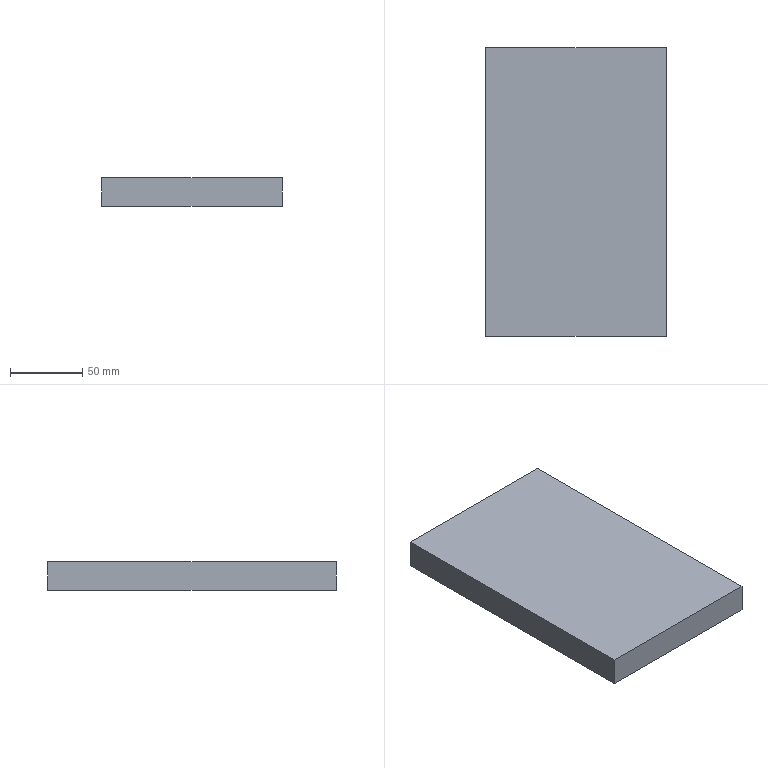Part | NX | features solid 2 | 1 solid | 6 faces | box 125 x 200 x 20 mm | volume 500000 mm3 | plane 6
STEP:
#1=CARTESIAN_POINT('',(-62.5,475.,-375.));
#2=VERTEX_POINT('',#1);
#3=CARTESIAN_POINT('',(-62.5,475.,-355.));
#4=VERTEX_POINT('',#3);
#5=CARTESIAN_POINT('',(-62.5,475.,-375.));
#6=DIRECTION('',(0.,0.,1.));
#7=VECTOR('',#6,1000.);
#8=LINE('',#5,#7);
#9=EDGE_CURVE('',#2,#4,#8,.T.);
#10=ORIENTED_EDGE('',*,*,#9,.F.);
#11=CARTESIAN_POINT('',(62.5,475.,-375.));
#12=VERTEX_POINT('',#11);
#13=CARTESIAN_POINT('',(75.,475.,-375.));
#14=DIRECTION('',(-1.,0.,0.));
#15=VECTOR('',#14,1000.);
#16=LINE('',#13,#15);
#17=EDGE_CURVE('',#12,#2,#16,.T.);
#18=ORIENTED_EDGE('',*,*,#17,.F.);
#19=CARTESIAN_POINT('',(62.5,475.,-355.));
#20=VERTEX_POINT('',#19);
#21=CARTESIAN_POINT('',(62.5,475.,-375.));
#22=DIRECTION('',(0.,0.,1.));
#23=VECTOR('',#22,1000.);
#24=LINE('',#21,#23);
#25=EDGE_CURVE('',#12,#20,#24,.T.);
#26=ORIENTED_EDGE('',*,*,#25,.T.);
#27=CARTESIAN_POINT('',(75.,475.,-355.));
#28=DIRECTION('',(-1.,0.,0.));
#29=VECTOR('',#28,1000.);
#30=LINE('',#27,#29);
#31=EDGE_CURVE('',#20,#4,#30,.T.);
#32=ORIENTED_EDGE('',*,*,#31,.T.);
#33=EDGE_LOOP('',(#10,#18,#26,#32));
#34=FACE_BOUND('',#33,.T.);
#35=CARTESIAN_POINT('',(75.,475.,-375.));
#36=DIRECTION('',(0.,-1.,0.));
#37=DIRECTION('',(0.,0.,-1.));
#38=AXIS2_PLACEMENT_3D('',#35,#36,#37);
#39=PLANE('',#38);
#40=ADVANCED_FACE('',(#34),#39,.T.);
#41=CARTESIAN_POINT('',(-62.5,675.,-375.));
#42=VERTEX_POINT('',#41);
#43=CARTESIAN_POINT('',(-62.5,675.,-375.));
#44=DIRECTION('',(0.,-1.,0.));
#45=VECTOR('',#44,1000.);
#46=LINE('',#43,#45);
#47=EDGE_CURVE('',#42,#2,#46,.T.);
#48=ORIENTED_EDGE('',*,*,#47,.F.);
#49=CARTESIAN_POINT('',(62.5,675.,-375.));
#50=VERTEX_POINT('',#49);
#51=CARTESIAN_POINT('',(75.,675.,-375.));
#52=DIRECTION('',(-1.,0.,0.));
#53=VECTOR('',#52,1000.);
#54=LINE('',#51,#53);
#55=EDGE_CURVE('',#50,#42,#54,.T.);
#56=ORIENTED_EDGE('',*,*,#55,.F.);
#57=CARTESIAN_POINT('',(62.5,675.,-375.));
#58=DIRECTION('',(0.,-1.,0.));
#59=VECTOR('',#58,1000.);
#60=LINE('',#57,#59);
#61=EDGE_CURVE('',#50,#12,#60,.T.);
#62=ORIENTED_EDGE('',*,*,#61,.T.);
#63=ORIENTED_EDGE('',*,*,#17,.T.);
#64=EDGE_LOOP('',(#48,#56,#62,#63));
#65=FACE_BOUND('',#64,.T.);
#66=CARTESIAN_POINT('',(75.,675.,-375.));
#67=DIRECTION('',(0.,0.,-1.));
#68=DIRECTION('',(-1.,0.,0.));
#69=AXIS2_PLACEMENT_3D('',#66,#67,#68);
#70=PLANE('',#69);
#71=ADVANCED_FACE('',(#65),#70,.T.);
#72=CARTESIAN_POINT('',(-62.5,675.,-355.));
#73=VERTEX_POINT('',#72);
#74=CARTESIAN_POINT('',(-62.5,675.,-375.));
#75=DIRECTION('',(0.,0.,1.));
#76=VECTOR('',#75,1000.);
#77=LINE('',#74,#76);
#78=EDGE_CURVE('',#42,#73,#77,.T.);
#79=ORIENTED_EDGE('',*,*,#78,.T.);
#80=CARTESIAN_POINT('',(62.5,675.,-355.));
#81=VERTEX_POINT('',#80);
#82=CARTESIAN_POINT('',(75.,675.,-355.));
#83=DIRECTION('',(-1.,0.,0.));
#84=VECTOR('',#83,1000.);
#85=LINE('',#82,#84);
#86=EDGE_CURVE('',#81,#73,#85,.T.);
#87=ORIENTED_EDGE('',*,*,#86,.F.);
#88=CARTESIAN_POINT('',(62.5,675.,-375.));
#89=DIRECTION('',(0.,0.,1.));
#90=VECTOR('',#89,1000.);
#91=LINE('',#88,#90);
#92=EDGE_CURVE('',#50,#81,#91,.T.);
#93=ORIENTED_EDGE('',*,*,#92,.F.);
#94=ORIENTED_EDGE('',*,*,#55,.T.);
#95=EDGE_LOOP('',(#79,#87,#93,#94));
#96=FACE_BOUND('',#95,.T.);
#97=CARTESIAN_POINT('',(75.,675.,-375.));
#98=DIRECTION('',(0.,-1.,0.));
#99=DIRECTION('',(0.,0.,-1.));
#100=AXIS2_PLACEMENT_3D('',#97,#98,#99);
#101=PLANE('',#100);
#102=ADVANCED_FACE('',(#96),#101,.F.);
#103=CARTESIAN_POINT('',(-62.5,690.404,-355.));
#104=DIRECTION('',(0.,-1.,0.));
#105=VECTOR('',#104,1000.);
#106=LINE('',#103,#105);
#107=EDGE_CURVE('',#73,#4,#106,.T.);
#108=ORIENTED_EDGE('',*,*,#107,.T.);
#109=ORIENTED_EDGE('',*,*,#31,.F.);
#110=CARTESIAN_POINT('',(62.5,690.404,-355.));
#111=DIRECTION('',(0.,-1.,0.));
#112=VECTOR('',#111,1000.);
#113=LINE('',#110,#112);
#114=EDGE_CURVE('',#81,#20,#113,.T.);
#115=ORIENTED_EDGE('',*,*,#114,.F.);
#116=ORIENTED_EDGE('',*,*,#86,.T.);
#117=EDGE_LOOP('',(#108,#109,#115,#116));
#118=FACE_BOUND('',#117,.T.);
#119=CARTESIAN_POINT('',(75.,690.404,-355.));
#120=DIRECTION('',(0.,0.,-1.));
#121=DIRECTION('',(-1.,0.,0.));
#122=AXIS2_PLACEMENT_3D('',#119,#120,#121);
#123=PLANE('',#122);
#124=ADVANCED_FACE('',(#118),#123,.F.);
#125=ORIENTED_EDGE('',*,*,#25,.F.);
#126=ORIENTED_EDGE('',*,*,#61,.F.);
#127=ORIENTED_EDGE('',*,*,#92,.T.);
#128=ORIENTED_EDGE('',*,*,#114,.T.);
#129=EDGE_LOOP('',(#125,#126,#127,#128));
#130=FACE_BOUND('',#129,.T.);
#131=CARTESIAN_POINT('',(62.5,628.851,-365.));
#132=DIRECTION('',(1.,0.,0.));
#133=DIRECTION('',(0.,0.,-1.));
#134=AXIS2_PLACEMENT_3D('',#131,#132,#133);
#135=PLANE('',#134);
#136=ADVANCED_FACE('',(#130),#135,.T.);
#137=ORIENTED_EDGE('',*,*,#9,.T.);
#138=ORIENTED_EDGE('',*,*,#107,.F.);
#139=ORIENTED_EDGE('',*,*,#78,.F.);
#140=ORIENTED_EDGE('',*,*,#47,.T.);
#141=EDGE_LOOP('',(#137,#138,#139,#140));
#142=FACE_BOUND('',#141,.T.);
#143=CARTESIAN_POINT('',(-62.5,628.851,-365.));
#144=DIRECTION('',(1.,0.,0.));
#145=DIRECTION('',(0.,0.,-1.));
#146=AXIS2_PLACEMENT_3D('',#143,#144,#145);
#147=PLANE('',#146);
#148=ADVANCED_FACE('',(#142),#147,.F.);
#149=CLOSED_SHELL('',(#40,#71,#102,#124,#136,#148));
#150=MANIFOLD_SOLID_BREP('',#149);
#151=(LENGTH_UNIT()NAMED_UNIT(*)SI_UNIT(.MILLI.,.METRE.));
#152=UNCERTAINTY_MEASURE_WITH_UNIT(LENGTH_MEASURE(0.00001),#151,'','');
#153=(NAMED_UNIT(*)PLANE_ANGLE_UNIT()SI_UNIT($,.RADIAN.));
#154=(NAMED_UNIT(*)SI_UNIT($,.STERADIAN.)SOLID_ANGLE_UNIT());
#155=(GEOMETRIC_REPRESENTATION_CONTEXT(3)GLOBAL_UNCERTAINTY_ASSIGNED_CONTEXT((#152))GLOBAL_UNIT_ASSIGNED_CONTEXT((#151,#153,#154))REPRESENTATION_CONTEXT('',''));
#156=ADVANCED_BREP_SHAPE_REPRESENTATION('',(#150),#155);